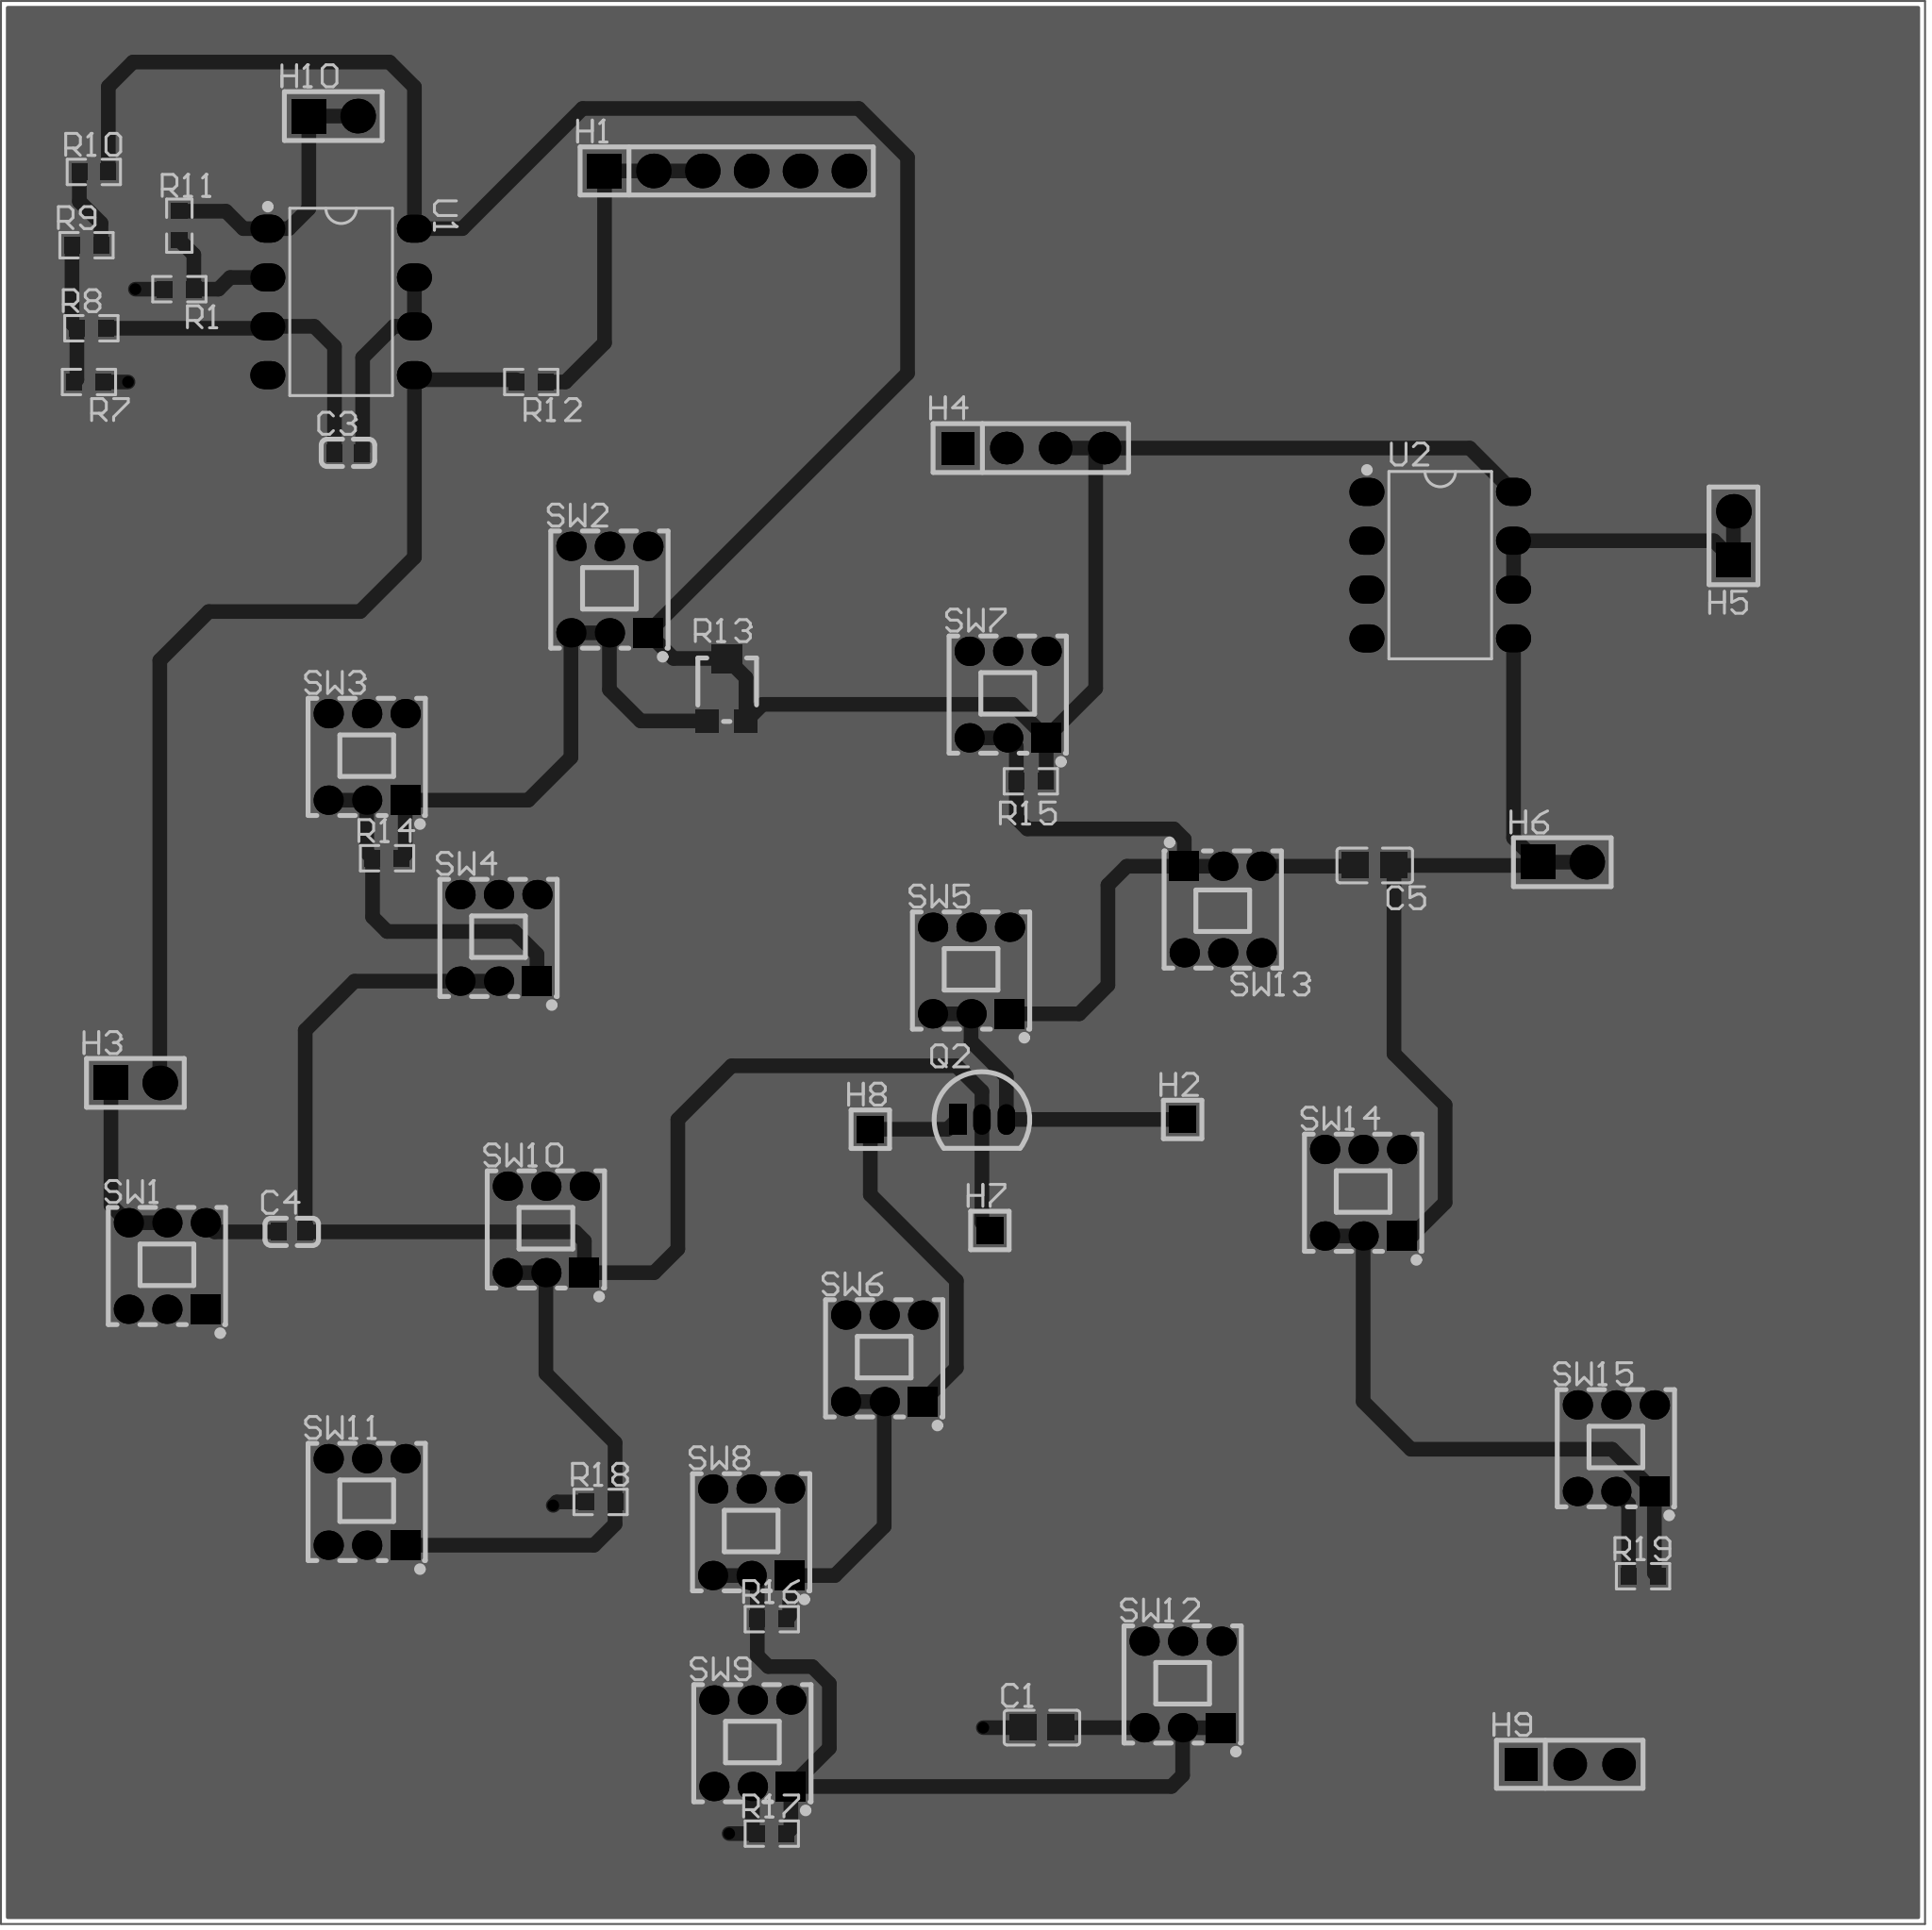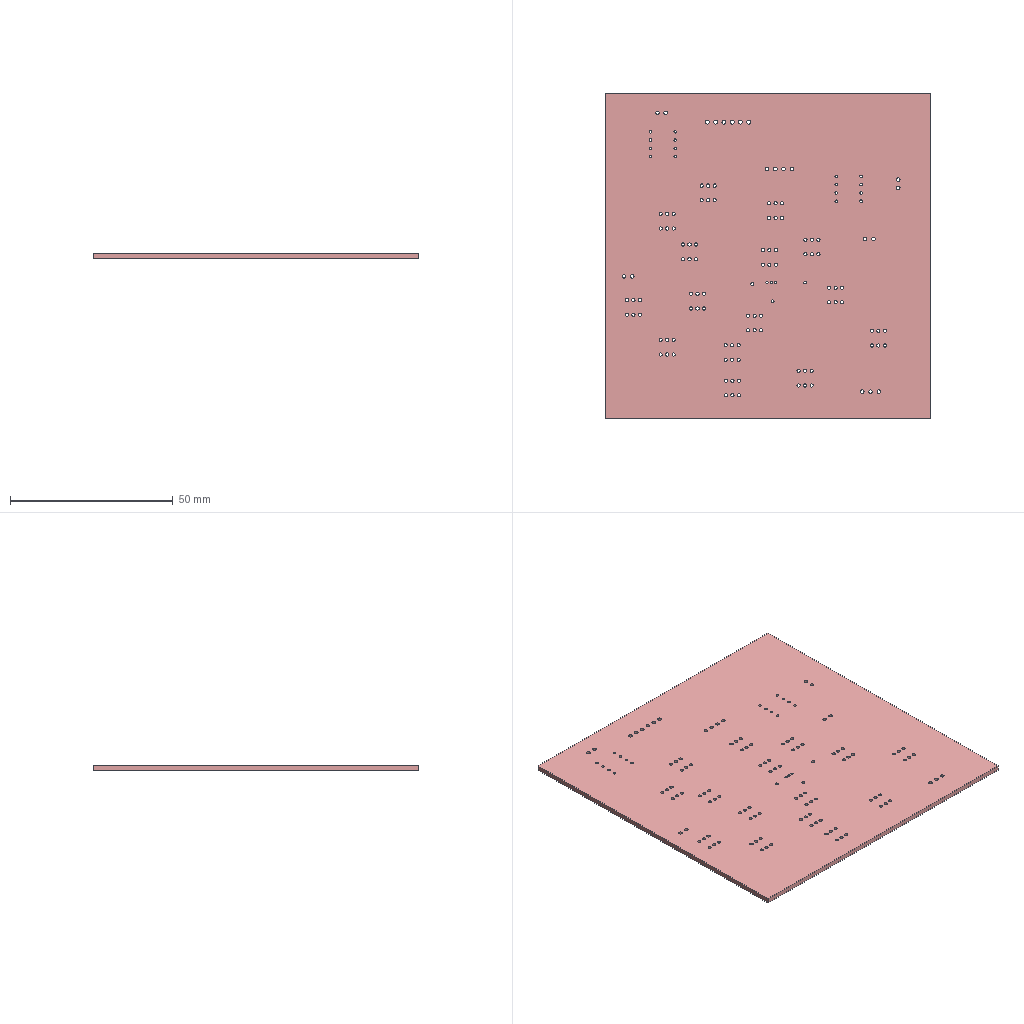Circuit board layout | Altium Designer | box 100 x 100 x 1.6 mm
Layer stack:
# Altium Designer layer stack of  (unit mm; dielectric type: 0 none, 1 core, 2 prepreg, 3 surface material)
index,name,kind,layer,copper_thickness_mm,dielectric_type,dielectric_thickness_mm,dielectric_material,dielectric_constant
0,Top Paste Mask Layer,other,,,,,,
1,Top Silkscreen Layer,other,,,,,,
2,Top Solder Mask Layer,dielectric,,,3,0.01,,3.3
3,Top Layer,copper,Top Layer,0.035,,,,
4,Dielectric1,dielectric,,,3,1.51,FR4,4.5
5,Bottom Layer,copper,Bottom Layer,0.035,,,,
6,Bottom Solder Mask Layer,dielectric,,,3,0.01,,3.3
7,Bottom Silkscreen Layer,other,,,,,,
8,Bottom Paste Mask Layer,other,,,,,,
# drill layer pairs: low layer,high layer
drill_pair,Top Layer,Bottom Layer
Part placement:
Designator,Comment,Layer,Footprint,Center-X(mm),Center-Y(mm),Rotation
C1,100uF,TopLayer,C0805,146.558,94.234,0
C3,0.47uF,TopLayer,C0603,110.49,160.528,0
C4,10uF,TopLayer,C0603,107.569,120.015,0
C5,10uF,TopLayer,C0805,163.855,139.069,180
H1,,TopLayer,HDR-TH_6P-P2.54-V-M-1,130.175,175.185,0
H2,,TopLayer,HDR-TH_1P-V-M_XKB_X4611WV-01I-C28D40,153.87,125.86,0
H3,,TopLayer,HDR-TH_2P-P2.54-V-M-1,99.441,127.762,0
H4,,TopLayer,HDR-TH_4P-P2.54-V-M,145.98,160.774,0
H5,,TopLayer,HDR-TH_2P-P2.54-V-M-1,182.499,156.21,90
H6,,TopLayer,HDR-TH_2P-P2.54-V-M-1,173.603,139.24,0
H7,,TopLayer,HDR-TH_1P-V-M_XKB_X4611WV-01I-C28D40,143.853,120.087,0
H8,,TopLayer,HDR-TH_1P-V-M_XKB_X4611WV-01I-C28D40,137.638,125.352,0
H9,,TopLayer,HDR-TH_3P-P2.54-V-M,173.99,92.329,0
H10,,TopLayer,HDR-TH_2P-P2.54-V-M-1,109.725,178.038,0
Q2,2N2222A,TopLayer,TO-92-3_L4.9-W3.7-P1.27-L,143.44,125.86,0
R1,1kΩ,TopLayer,R0603,101.727,169.037,180
R7,1kΩ,TopLayer,R0603,97.028,164.211,180
R8,2kΩ,TopLayer,R0603,97.155,167.005,0
R9,100kΩ,TopLayer,R0603,96.901,171.323,0
R10,100kΩ,TopLayer,R0603,97.282,175.133,0
R11,20kΩ,TopLayer,R0603,101.727,172.339,90
R12,10KΩ,TopLayer,R0603,120.015,164.211,180
R13,100kΩ,TopLayer,RES-ADJ-SMD_JER33X-1-14,130.175,148.209,0
R14,39kΩ,TopLayer,R0603,112.522,139.446,0
R15,24kΩ,TopLayer,R0603,145.98,143.444,0
R16,100Ω,TopLayer,R0603,132.518,99.874,0
R17,1kΩ,TopLayer,R0603,132.518,88.723,0
R18,20KΩ,TopLayer,R0603,123.62,105.97,0
R19,2.4KΩ,TopLayer,R0603,177.8,102.108,0
SW1,5.8 ZSGT,TopLayer,SW-TH_5.8ZSGT,101.081,118.24,0
SW2,5.8 ZSGT,TopLayer,SW-TH_5.8ZSGT,124.079,153.416,0
SW3,5.8 ZSGT,TopLayer,SW-TH_5.8ZSGT,111.465,144.714,0
SW4,5.8 ZSGT,TopLayer,SW-TH_5.8ZSGT,118.315,135.303,0
SW5,5.8 ZSGT,TopLayer,SW-TH_5.8ZSGT,142.875,133.604,0
SW6,5.8 ZSGT,TopLayer,SW-TH_5.8ZSGT,138.36,113.438,0
SW7,5.8 ZSGT,TopLayer,SW-TH_5.8ZSGT,144.78,147.955,0
SW8,5.8 ZSGT,TopLayer,SW-TH_5.8ZSGT,131.445,104.394,0
SW9,5.8 ZSGT,TopLayer,SW-TH_5.8ZSGT,131.51,93.422,0
SW10,5.8 ZSGT,TopLayer,SW-TH_5.8ZSGT,120.777,120.142,0
SW11,5.8 ZSGT,TopLayer,SW-TH_5.8ZSGT,111.465,105.97,0
SW12,5.8 ZSGT,TopLayer,SW-TH_5.8ZSGT,153.87,96.479,0
SW13,5.8 ZSGT,TopLayer,SW-TH_5.8ZSGT,155.956,136.779,180
SW14,5.8 ZSGT,TopLayer,SW-TH_5.8ZSGT,163.252,122.05,0
SW15,5.8 ZSGT,TopLayer,SW-TH_5.8ZSGT,176.389,108.764,0
U1,LM358P,TopLayer,DIP-8_L9.4-W6.4-P2.54-LS9.1-BL,110.135,168.376,270
U2,LM358P,TopLayer,DIP-8_L9.4-W6.4-P2.54-LS9.1-BL,167.259,154.686,270
Pad and via stacks:
# Altium Designer via and pad stacks of  (unit mm). Each distinct definition once, with the count of objects using it.
# via: kind,start_layer,end_layer,hole_mm,diameter_mm,mode(0 simple;1 top-mid-bottom;2 full stack),diameter_per_layer,count,example_net
# pad: kind,layer,hole_mm,hole_type(0 round;1 square;2 slot),plating,top_size,top_shape(1 round;2 rect;3 octagon;9 rounded rect),mid_size,bottom_size,mode,footprint,size_per_layer,count,example
pad,Top Layer,0,0,plated,1.41x1.35,2,1.41x1.35,1.41x1.35,0,C0805,,4,C1.2
pad,Top Layer,0,0,plated,0.8x0.9,2,0.8x0.9,0.8x0.9,0,C0603,,4,C3.2
pad,Top Layer,0,0,plated,0.8065x0.864,2,0.8065x0.864,0.8065x0.864,0,R0603,,26,R1.2
pad,Top Layer,0,0,plated,1.2x1.2,2,1.2x1.2,1.2x1.2,0,RES-ADJ-SMD_JER33X-1-14,,2,R13.1
pad,Top Layer,0,0,plated,1.5x1.6,2,1.5x1.6,1.5x1.6,0,RES-ADJ-SMD_JER33X-1-14,,1,R13.2
pad,Multi-Layer,1.2,0,plated,1.8x1.8,1,1.8x1.8,1.8x1.8,0,HDR-TH_6P-P2.54-V-M-1,,5,H1.6
pad,Multi-Layer,1.2,0,plated,1.8x1.8,2,1.8x1.8,1.8x1.8,0,HDR-TH_6P-P2.54-V-M-1,,1,H1.1
pad,Multi-Layer,0.9,0,plated,1.4x1.4,2,1.4x1.4,1.4x1.4,0,HDR-TH_1P-V-M_XKB_X4611WV-01I-C28D40,,3,H2.1
pad,Multi-Layer,1.1,0,plated,1.8x1.8,1,1.8x1.8,1.8x1.8,0,HDR-TH_2P-P2.54-V-M-1,,4,H3.2
pad,Multi-Layer,1.1,0,plated,1.8x1.8,2,1.8x1.8,1.8x1.8,0,HDR-TH_2P-P2.54-V-M-1,,4,H3.1
pad,Multi-Layer,1.1,0,plated,1.7x1.7,2,1.7x1.7,1.7x1.7,0,HDR-TH_4P-P2.54-V-M,,1,H4.1
pad,Multi-Layer,1.1,0,plated,1.7x1.7,1,1.7x1.7,1.7x1.7,0,HDR-TH_4P-P2.54-V-M,,3,H4.2
pad,Multi-Layer,1.1,0,plated,1.7x1.7,2,1.7x1.7,1.7x1.7,0,HDR-TH_3P-P2.54-V-M,,1,H9.1
pad,Multi-Layer,1.1,0,plated,1.7x1.7,1,1.7x1.7,1.7x1.7,0,HDR-TH_3P-P2.54-V-M,,2,H9.2
pad,Multi-Layer,0.7,0,plated,0.9x1.6,1,0.9x1.6,0.9x1.6,0,TO-92-3_L4.9-W3.7-P1.27-L,,2,Q2.3
pad,Multi-Layer,0.7,0,plated,0.9x1.6,2,0.9x1.6,0.9x1.6,0,TO-92-3_L4.9-W3.7-P1.27-L,,1,Q2.1
pad,Multi-Layer,1,0,plated,1.524x1.524,1,1.524x1.524,1.524x1.524,0,SW-TH_5.8ZSGT,,75,SW1.4
pad,Multi-Layer,1,0,plated,1.524x1.524,2,1.524x1.524,1.524x1.524,0,SW-TH_5.8ZSGT,,15,SW1.1
pad,Multi-Layer,0.8,0,plated,1.46x1.825,1,1.46x1.825,1.46x1.825,0,DIP-8_L9.4-W6.4-P2.54-LS9.1-BL,,16,U1.1
via,Top Layer,Bottom Layer,0.3048,0.61,0,,5,GND
Copper pours:
name,layer,net,type(0 solid;1 hatched;2 none)
Bottom Layer-GND,Bottom Layer,GND,0
Design rules, without the lines most boards share:
# Altium Designer design rules of  (exported by Altium Designer, unit mm)
# columns: name | kind | enabled | priority | scope1 | scope2 | descriptor | typed fields (field=value)
creepage | 65 | enabled | 1 | All | All | Creepage Distance Constraint =(0mil) (All),(All) |